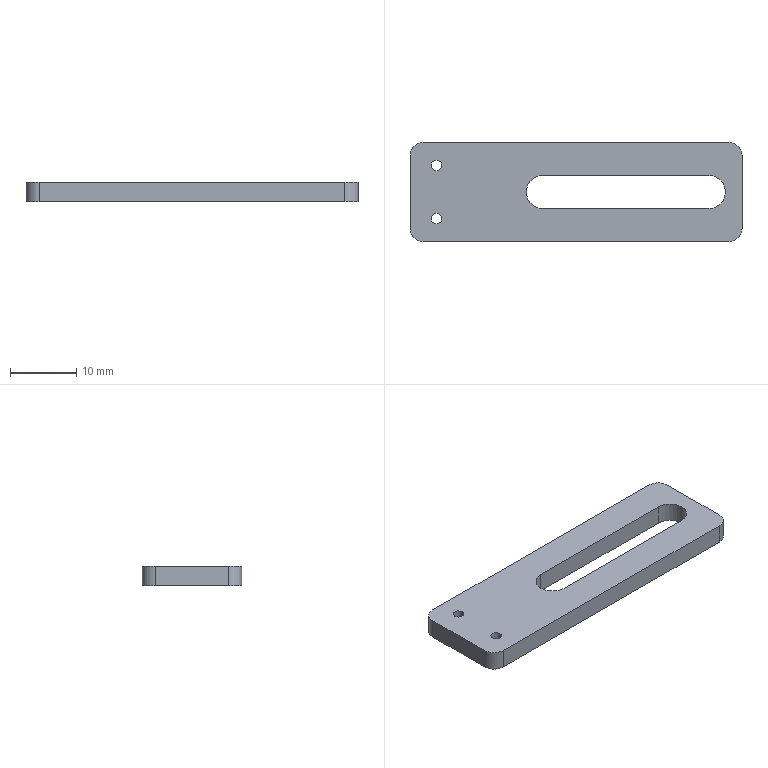Part | STEP file | 1004-2001-0085_1004-2001-0085_1-2 | 1 solid | 19 faces | box 50 x 15 x 3 mm | volume 1794 mm3 | cylinder 11 | plane 8 | commonest cylinder face diameters 1.6 x4 4 x4 5 x3
STEP:
#1=CARTESIAN_POINT('',(-20.2,-4.,1.5));
#2=VERTEX_POINT('',#1);
#3=CARTESIAN_POINT('',(-21.8,-4.,1.5));
#4=VERTEX_POINT('',#3);
#5=CARTESIAN_POINT('',(-21.,-4.,1.5));
#6=DIRECTION('',(0.,0.,-1.));
#7=DIRECTION('',(-1.,0.,0.));
#8=AXIS2_PLACEMENT_3D('',#5,#6,#7);
#9=CIRCLE('',#8,0.8);
#10=EDGE_CURVE('',#2,#4,#9,.T.);
#11=ORIENTED_EDGE('',*,*,#10,.F.);
#12=CARTESIAN_POINT('',(-20.2,-4.,-1.5));
#13=VERTEX_POINT('',#12);
#14=CARTESIAN_POINT('',(-20.2,-4.,-1.5));
#15=DIRECTION('',(0.,0.,-1.));
#16=VECTOR('',#15,1000.);
#17=LINE('',#14,#16);
#18=EDGE_CURVE('',#2,#13,#17,.T.);
#19=ORIENTED_EDGE('',*,*,#18,.T.);
#20=CARTESIAN_POINT('',(-21.8,-4.,-1.5));
#21=VERTEX_POINT('',#20);
#22=CARTESIAN_POINT('',(-21.,-4.,-1.5));
#23=DIRECTION('',(0.,0.,1.));
#24=DIRECTION('',(-1.,0.,0.));
#25=AXIS2_PLACEMENT_3D('',#22,#23,#24);
#26=CIRCLE('',#25,0.8);
#27=EDGE_CURVE('',#21,#13,#26,.T.);
#28=ORIENTED_EDGE('',*,*,#27,.F.);
#29=CARTESIAN_POINT('',(-21.8,-4.,-1.5));
#30=DIRECTION('',(0.,0.,-1.));
#31=VECTOR('',#30,1000.);
#32=LINE('',#29,#31);
#33=EDGE_CURVE('',#4,#21,#32,.T.);
#34=ORIENTED_EDGE('',*,*,#33,.F.);
#35=EDGE_LOOP('',(#11,#19,#28,#34));
#36=FACE_OUTER_BOUND('',#35,.T.);
#37=CARTESIAN_POINT('',(-21.,-4.,-1.5));
#38=DIRECTION('',(0.,0.,-1.));
#39=DIRECTION('',(-1.,0.,0.));
#40=AXIS2_PLACEMENT_3D('',#37,#38,#39);
#41=CYLINDRICAL_SURFACE('',#40,0.8);
#42=ADVANCED_FACE('',(#36),#41,.F.);
#43=CARTESIAN_POINT('',(-20.2,4.,1.5));
#44=VERTEX_POINT('',#43);
#45=CARTESIAN_POINT('',(-21.8,4.,1.5));
#46=VERTEX_POINT('',#45);
#47=CARTESIAN_POINT('',(-21.,4.,1.5));
#48=DIRECTION('',(0.,0.,-1.));
#49=DIRECTION('',(-1.,0.,0.));
#50=AXIS2_PLACEMENT_3D('',#47,#48,#49);
#51=CIRCLE('',#50,0.8);
#52=EDGE_CURVE('',#44,#46,#51,.T.);
#53=ORIENTED_EDGE('',*,*,#52,.F.);
#54=CARTESIAN_POINT('',(-20.2,4.,-1.5));
#55=VERTEX_POINT('',#54);
#56=CARTESIAN_POINT('',(-20.2,4.,-1.5));
#57=DIRECTION('',(0.,0.,-1.));
#58=VECTOR('',#57,1000.);
#59=LINE('',#56,#58);
#60=EDGE_CURVE('',#44,#55,#59,.T.);
#61=ORIENTED_EDGE('',*,*,#60,.T.);
#62=CARTESIAN_POINT('',(-21.8,4.,-1.5));
#63=VERTEX_POINT('',#62);
#64=CARTESIAN_POINT('',(-21.,4.,-1.5));
#65=DIRECTION('',(0.,0.,1.));
#66=DIRECTION('',(-1.,0.,0.));
#67=AXIS2_PLACEMENT_3D('',#64,#65,#66);
#68=CIRCLE('',#67,0.8);
#69=EDGE_CURVE('',#63,#55,#68,.T.);
#70=ORIENTED_EDGE('',*,*,#69,.F.);
#71=CARTESIAN_POINT('',(-21.8,4.,-1.5));
#72=DIRECTION('',(0.,0.,-1.));
#73=VECTOR('',#72,1000.);
#74=LINE('',#71,#73);
#75=EDGE_CURVE('',#46,#63,#74,.T.);
#76=ORIENTED_EDGE('',*,*,#75,.F.);
#77=EDGE_LOOP('',(#53,#61,#70,#76));
#78=FACE_OUTER_BOUND('',#77,.T.);
#79=CARTESIAN_POINT('',(-21.,4.,-1.5));
#80=DIRECTION('',(0.,0.,-1.));
#81=DIRECTION('',(-1.,0.,0.));
#82=AXIS2_PLACEMENT_3D('',#79,#80,#81);
#83=CYLINDRICAL_SURFACE('',#82,0.8);
#84=ADVANCED_FACE('',(#78),#83,.F.);
#85=CARTESIAN_POINT('',(-7.5,0.,1.5));
#86=VERTEX_POINT('',#85);
#87=CARTESIAN_POINT('',(-5.,2.5,1.5));
#88=VERTEX_POINT('',#87);
#89=CARTESIAN_POINT('',(-5.,0.,1.5));
#90=DIRECTION('',(0.,0.,-1.));
#91=DIRECTION('',(-1.,0.,0.));
#92=AXIS2_PLACEMENT_3D('',#89,#90,#91);
#93=CIRCLE('',#92,2.5);
#94=EDGE_CURVE('',#86,#88,#93,.T.);
#95=ORIENTED_EDGE('',*,*,#94,.F.);
#96=CARTESIAN_POINT('',(-7.5,0.,-1.5));
#97=VERTEX_POINT('',#96);
#98=CARTESIAN_POINT('',(-7.5,0.,1.5));
#99=DIRECTION('',(0.,0.,-1.));
#100=VECTOR('',#99,1000.);
#101=LINE('',#98,#100);
#102=EDGE_CURVE('',#86,#97,#101,.T.);
#103=ORIENTED_EDGE('',*,*,#102,.T.);
#104=CARTESIAN_POINT('',(-5.,2.5,-1.5));
#105=VERTEX_POINT('',#104);
#106=CARTESIAN_POINT('',(-5.,0.,-1.5));
#107=DIRECTION('',(0.,0.,1.));
#108=DIRECTION('',(-1.,0.,0.));
#109=AXIS2_PLACEMENT_3D('',#106,#107,#108);
#110=CIRCLE('',#109,2.5);
#111=EDGE_CURVE('',#105,#97,#110,.T.);
#112=ORIENTED_EDGE('',*,*,#111,.F.);
#113=CARTESIAN_POINT('',(-5.,2.5,1.5));
#114=DIRECTION('',(0.,0.,1.));
#115=VECTOR('',#114,1000.);
#116=LINE('',#113,#115);
#117=EDGE_CURVE('',#105,#88,#116,.T.);
#118=ORIENTED_EDGE('',*,*,#117,.T.);
#119=EDGE_LOOP('',(#95,#103,#112,#118));
#120=FACE_OUTER_BOUND('',#119,.T.);
#121=CARTESIAN_POINT('',(-5.,0.,1.5));
#122=DIRECTION('',(0.,0.,-1.));
#123=DIRECTION('',(-1.,0.,0.));
#124=AXIS2_PLACEMENT_3D('',#121,#122,#123);
#125=CYLINDRICAL_SURFACE('',#124,2.5);
#126=ADVANCED_FACE('',(#120),#125,.F.);
#127=CARTESIAN_POINT('',(-21.,-4.,1.5));
#128=DIRECTION('',(0.,0.,-1.));
#129=DIRECTION('',(-1.,0.,0.));
#130=AXIS2_PLACEMENT_3D('',#127,#128,#129);
#131=CIRCLE('',#130,0.8);
#132=EDGE_CURVE('',#4,#2,#131,.T.);
#133=ORIENTED_EDGE('',*,*,#132,.T.);
#134=ORIENTED_EDGE('',*,*,#10,.T.);
#135=EDGE_LOOP('',(#133,#134));
#136=FACE_BOUND('',#135,.T.);
#137=CARTESIAN_POINT('',(-21.,4.,1.5));
#138=DIRECTION('',(0.,0.,-1.));
#139=DIRECTION('',(-1.,0.,0.));
#140=AXIS2_PLACEMENT_3D('',#137,#138,#139);
#141=CIRCLE('',#140,0.8);
#142=EDGE_CURVE('',#46,#44,#141,.T.);
#143=ORIENTED_EDGE('',*,*,#142,.T.);
#144=ORIENTED_EDGE('',*,*,#52,.T.);
#145=EDGE_LOOP('',(#143,#144));
#146=FACE_BOUND('',#145,.T.);
#147=CARTESIAN_POINT('',(20.,-2.5,1.5));
#148=VERTEX_POINT('',#147);
#149=CARTESIAN_POINT('',(-5.,-2.5,1.5));
#150=VERTEX_POINT('',#149);
#151=CARTESIAN_POINT('',(-25.,-2.5,1.5));
#152=DIRECTION('',(-1.,0.,0.));
#153=VECTOR('',#152,1000.);
#154=LINE('',#151,#153);
#155=EDGE_CURVE('',#148,#150,#154,.T.);
#156=ORIENTED_EDGE('',*,*,#155,.T.);
#157=CARTESIAN_POINT('',(-5.,0.,1.5));
#158=DIRECTION('',(0.,0.,-1.));
#159=DIRECTION('',(-1.,0.,0.));
#160=AXIS2_PLACEMENT_3D('',#157,#158,#159);
#161=CIRCLE('',#160,2.5);
#162=EDGE_CURVE('',#150,#86,#161,.T.);
#163=ORIENTED_EDGE('',*,*,#162,.T.);
#164=ORIENTED_EDGE('',*,*,#94,.T.);
#165=CARTESIAN_POINT('',(20.,2.5,1.5));
#166=VERTEX_POINT('',#165);
#167=CARTESIAN_POINT('',(-25.,2.5,1.5));
#168=DIRECTION('',(1.,0.,0.));
#169=VECTOR('',#168,1000.);
#170=LINE('',#167,#169);
#171=EDGE_CURVE('',#88,#166,#170,.T.);
#172=ORIENTED_EDGE('',*,*,#171,.T.);
#173=CARTESIAN_POINT('',(20.,0.,1.5));
#174=DIRECTION('',(0.,0.,-1.));
#175=DIRECTION('',(-1.,0.,0.));
#176=AXIS2_PLACEMENT_3D('',#173,#174,#175);
#177=CIRCLE('',#176,2.5);
#178=EDGE_CURVE('',#166,#148,#177,.T.);
#179=ORIENTED_EDGE('',*,*,#178,.T.);
#180=EDGE_LOOP('',(#156,#163,#164,#172,#179));
#181=FACE_BOUND('',#180,.T.);
#182=CARTESIAN_POINT('',(23.,-7.5,1.5));
#183=VERTEX_POINT('',#182);
#184=CARTESIAN_POINT('',(25.,-5.5,1.5));
#185=VERTEX_POINT('',#184);
#186=CARTESIAN_POINT('',(23.,-5.5,1.5));
#187=DIRECTION('',(0.,0.,1.));
#188=DIRECTION('',(-1.,0.,0.));
#189=AXIS2_PLACEMENT_3D('',#186,#187,#188);
#190=CIRCLE('',#189,2.);
#191=EDGE_CURVE('',#183,#185,#190,.T.);
#192=ORIENTED_EDGE('',*,*,#191,.T.);
#193=CARTESIAN_POINT('',(25.,5.5,1.5));
#194=VERTEX_POINT('',#193);
#195=CARTESIAN_POINT('',(25.,7.5,1.5));
#196=DIRECTION('',(0.,1.,0.));
#197=VECTOR('',#196,1000.);
#198=LINE('',#195,#197);
#199=EDGE_CURVE('',#185,#194,#198,.T.);
#200=ORIENTED_EDGE('',*,*,#199,.T.);
#201=CARTESIAN_POINT('',(23.,7.5,1.5));
#202=VERTEX_POINT('',#201);
#203=CARTESIAN_POINT('',(23.,5.5,1.5));
#204=DIRECTION('',(0.,0.,1.));
#205=DIRECTION('',(-1.,0.,0.));
#206=AXIS2_PLACEMENT_3D('',#203,#204,#205);
#207=CIRCLE('',#206,2.);
#208=EDGE_CURVE('',#194,#202,#207,.T.);
#209=ORIENTED_EDGE('',*,*,#208,.T.);
#210=CARTESIAN_POINT('',(-23.,7.5,1.5));
#211=VERTEX_POINT('',#210);
#212=CARTESIAN_POINT('',(-25.,7.5,1.5));
#213=DIRECTION('',(-1.,0.,0.));
#214=VECTOR('',#213,1000.);
#215=LINE('',#212,#214);
#216=EDGE_CURVE('',#202,#211,#215,.T.);
#217=ORIENTED_EDGE('',*,*,#216,.T.);
#218=CARTESIAN_POINT('',(-25.,5.5,1.5));
#219=VERTEX_POINT('',#218);
#220=CARTESIAN_POINT('',(-23.,5.5,1.5));
#221=DIRECTION('',(0.,0.,1.));
#222=DIRECTION('',(-1.,0.,0.));
#223=AXIS2_PLACEMENT_3D('',#220,#221,#222);
#224=CIRCLE('',#223,2.);
#225=EDGE_CURVE('',#211,#219,#224,.T.);
#226=ORIENTED_EDGE('',*,*,#225,.T.);
#227=CARTESIAN_POINT('',(-25.,-5.5,1.5));
#228=VERTEX_POINT('',#227);
#229=CARTESIAN_POINT('',(-25.,7.5,1.5));
#230=DIRECTION('',(0.,-1.,0.));
#231=VECTOR('',#230,1000.);
#232=LINE('',#229,#231);
#233=EDGE_CURVE('',#219,#228,#232,.T.);
#234=ORIENTED_EDGE('',*,*,#233,.T.);
#235=CARTESIAN_POINT('',(-23.,-7.5,1.5));
#236=VERTEX_POINT('',#235);
#237=CARTESIAN_POINT('',(-23.,-5.5,1.5));
#238=DIRECTION('',(0.,0.,1.));
#239=DIRECTION('',(-1.,0.,0.));
#240=AXIS2_PLACEMENT_3D('',#237,#238,#239);
#241=CIRCLE('',#240,2.);
#242=EDGE_CURVE('',#228,#236,#241,.T.);
#243=ORIENTED_EDGE('',*,*,#242,.T.);
#244=CARTESIAN_POINT('',(-25.,-7.5,1.5));
#245=DIRECTION('',(1.,0.,0.));
#246=VECTOR('',#245,1000.);
#247=LINE('',#244,#246);
#248=EDGE_CURVE('',#236,#183,#247,.T.);
#249=ORIENTED_EDGE('',*,*,#248,.T.);
#250=EDGE_LOOP('',(#192,#200,#209,#217,#226,#234,#243,#249));
#251=FACE_OUTER_BOUND('',#250,.T.);
#252=CARTESIAN_POINT('',(-25.,7.5,1.5));
#253=DIRECTION('',(0.,0.,1.));
#254=DIRECTION('',(1.,0.,0.));
#255=AXIS2_PLACEMENT_3D('',#252,#253,#254);
#256=PLANE('',#255);
#257=ADVANCED_FACE('',(#136,#146,#181,#251),#256,.T.);
#258=ORIENTED_EDGE('',*,*,#18,.F.);
#259=ORIENTED_EDGE('',*,*,#132,.F.);
#260=ORIENTED_EDGE('',*,*,#33,.T.);
#261=CARTESIAN_POINT('',(-21.,-4.,-1.5));
#262=DIRECTION('',(0.,0.,1.));
#263=DIRECTION('',(-1.,0.,0.));
#264=AXIS2_PLACEMENT_3D('',#261,#262,#263);
#265=CIRCLE('',#264,0.8);
#266=EDGE_CURVE('',#13,#21,#265,.T.);
#267=ORIENTED_EDGE('',*,*,#266,.F.);
#268=EDGE_LOOP('',(#258,#259,#260,#267));
#269=FACE_OUTER_BOUND('',#268,.T.);
#270=CARTESIAN_POINT('',(-21.,-4.,-1.5));
#271=DIRECTION('',(0.,0.,-1.));
#272=DIRECTION('',(-1.,0.,0.));
#273=AXIS2_PLACEMENT_3D('',#270,#271,#272);
#274=CYLINDRICAL_SURFACE('',#273,0.8);
#275=ADVANCED_FACE('',(#269),#274,.F.);
#276=ORIENTED_EDGE('',*,*,#60,.F.);
#277=ORIENTED_EDGE('',*,*,#142,.F.);
#278=ORIENTED_EDGE('',*,*,#75,.T.);
#279=CARTESIAN_POINT('',(-21.,4.,-1.5));
#280=DIRECTION('',(0.,0.,1.));
#281=DIRECTION('',(-1.,0.,0.));
#282=AXIS2_PLACEMENT_3D('',#279,#280,#281);
#283=CIRCLE('',#282,0.8);
#284=EDGE_CURVE('',#55,#63,#283,.T.);
#285=ORIENTED_EDGE('',*,*,#284,.F.);
#286=EDGE_LOOP('',(#276,#277,#278,#285));
#287=FACE_OUTER_BOUND('',#286,.T.);
#288=CARTESIAN_POINT('',(-21.,4.,-1.5));
#289=DIRECTION('',(0.,0.,-1.));
#290=DIRECTION('',(-1.,0.,0.));
#291=AXIS2_PLACEMENT_3D('',#288,#289,#290);
#292=CYLINDRICAL_SURFACE('',#291,0.8);
#293=ADVANCED_FACE('',(#287),#292,.F.);
#294=ORIENTED_EDGE('',*,*,#102,.F.);
#295=ORIENTED_EDGE('',*,*,#162,.F.);
#296=CARTESIAN_POINT('',(-5.,-2.5,-1.5));
#297=VERTEX_POINT('',#296);
#298=CARTESIAN_POINT('',(-5.,-2.5,1.5));
#299=DIRECTION('',(0.,0.,1.));
#300=VECTOR('',#299,1000.);
#301=LINE('',#298,#300);
#302=EDGE_CURVE('',#297,#150,#301,.T.);
#303=ORIENTED_EDGE('',*,*,#302,.F.);
#304=CARTESIAN_POINT('',(-5.,0.,-1.5));
#305=DIRECTION('',(0.,0.,1.));
#306=DIRECTION('',(-1.,0.,0.));
#307=AXIS2_PLACEMENT_3D('',#304,#305,#306);
#308=CIRCLE('',#307,2.5);
#309=EDGE_CURVE('',#97,#297,#308,.T.);
#310=ORIENTED_EDGE('',*,*,#309,.F.);
#311=EDGE_LOOP('',(#294,#295,#303,#310));
#312=FACE_OUTER_BOUND('',#311,.T.);
#313=CARTESIAN_POINT('',(-5.,0.,1.5));
#314=DIRECTION('',(0.,0.,-1.));
#315=DIRECTION('',(-1.,0.,0.));
#316=AXIS2_PLACEMENT_3D('',#313,#314,#315);
#317=CYLINDRICAL_SURFACE('',#316,2.5);
#318=ADVANCED_FACE('',(#312),#317,.F.);
#319=ORIENTED_EDGE('',*,*,#155,.F.);
#320=CARTESIAN_POINT('',(20.,-2.5,-1.5));
#321=VERTEX_POINT('',#320);
#322=CARTESIAN_POINT('',(20.,-2.5,1.5));
#323=DIRECTION('',(0.,0.,1.));
#324=VECTOR('',#323,1000.);
#325=LINE('',#322,#324);
#326=EDGE_CURVE('',#321,#148,#325,.T.);
#327=ORIENTED_EDGE('',*,*,#326,.F.);
#328=CARTESIAN_POINT('',(-5.,-2.5,-1.5));
#329=DIRECTION('',(1.,0.,0.));
#330=VECTOR('',#329,1000.);
#331=LINE('',#328,#330);
#332=EDGE_CURVE('',#297,#321,#331,.T.);
#333=ORIENTED_EDGE('',*,*,#332,.F.);
#334=ORIENTED_EDGE('',*,*,#302,.T.);
#335=EDGE_LOOP('',(#319,#327,#333,#334));
#336=FACE_OUTER_BOUND('',#335,.T.);
#337=CARTESIAN_POINT('',(-5.,-2.5,1.5));
#338=DIRECTION('',(0.,-1.,0.));
#339=DIRECTION('',(0.,0.,-1.));
#340=AXIS2_PLACEMENT_3D('',#337,#338,#339);
#341=PLANE('',#340);
#342=ADVANCED_FACE('',(#336),#341,.F.);
#343=ORIENTED_EDGE('',*,*,#326,.T.);
#344=ORIENTED_EDGE('',*,*,#178,.F.);
#345=CARTESIAN_POINT('',(20.,2.5,-1.5));
#346=VERTEX_POINT('',#345);
#347=CARTESIAN_POINT('',(20.,2.5,1.5));
#348=DIRECTION('',(0.,0.,1.));
#349=VECTOR('',#348,1000.);
#350=LINE('',#347,#349);
#351=EDGE_CURVE('',#346,#166,#350,.T.);
#352=ORIENTED_EDGE('',*,*,#351,.F.);
#353=CARTESIAN_POINT('',(20.,0.,-1.5));
#354=DIRECTION('',(0.,0.,1.));
#355=DIRECTION('',(-1.,0.,0.));
#356=AXIS2_PLACEMENT_3D('',#353,#354,#355);
#357=CIRCLE('',#356,2.5);
#358=EDGE_CURVE('',#321,#346,#357,.T.);
#359=ORIENTED_EDGE('',*,*,#358,.F.);
#360=EDGE_LOOP('',(#343,#344,#352,#359));
#361=FACE_OUTER_BOUND('',#360,.T.);
#362=CARTESIAN_POINT('',(20.,0.,1.5));
#363=DIRECTION('',(0.,0.,-1.));
#364=DIRECTION('',(-1.,0.,0.));
#365=AXIS2_PLACEMENT_3D('',#362,#363,#364);
#366=CYLINDRICAL_SURFACE('',#365,2.5);
#367=ADVANCED_FACE('',(#361),#366,.F.);
#368=ORIENTED_EDGE('',*,*,#171,.F.);
#369=ORIENTED_EDGE('',*,*,#117,.F.);
#370=CARTESIAN_POINT('',(-5.,2.5,-1.5));
#371=DIRECTION('',(-1.,0.,0.));
#372=VECTOR('',#371,1000.);
#373=LINE('',#370,#372);
#374=EDGE_CURVE('',#346,#105,#373,.T.);
#375=ORIENTED_EDGE('',*,*,#374,.F.);
#376=ORIENTED_EDGE('',*,*,#351,.T.);
#377=EDGE_LOOP('',(#368,#369,#375,#376));
#378=FACE_OUTER_BOUND('',#377,.T.);
#379=CARTESIAN_POINT('',(-5.,2.5,1.5));
#380=DIRECTION('',(0.,1.,0.));
#381=DIRECTION('',(0.,0.,1.));
#382=AXIS2_PLACEMENT_3D('',#379,#380,#381);
#383=PLANE('',#382);
#384=ADVANCED_FACE('',(#378),#383,.F.);
#385=ORIENTED_EDGE('',*,*,#199,.F.);
#386=CARTESIAN_POINT('',(25.,-5.5,-1.5));
#387=VERTEX_POINT('',#386);
#388=CARTESIAN_POINT('',(25.,-5.5,1.5));
#389=DIRECTION('',(0.,0.,1.));
#390=VECTOR('',#389,1000.);
#391=LINE('',#388,#390);
#392=EDGE_CURVE('',#387,#185,#391,.T.);
#393=ORIENTED_EDGE('',*,*,#392,.F.);
#394=CARTESIAN_POINT('',(25.,5.5,-1.5));
#395=VERTEX_POINT('',#394);
#396=CARTESIAN_POINT('',(25.,-7.5,-1.5));
#397=DIRECTION('',(0.,-1.,0.));
#398=VECTOR('',#397,1000.);
#399=LINE('',#396,#398);
#400=EDGE_CURVE('',#395,#387,#399,.T.);
#401=ORIENTED_EDGE('',*,*,#400,.F.);
#402=CARTESIAN_POINT('',(25.,5.5,1.5));
#403=DIRECTION('',(0.,0.,-1.));
#404=VECTOR('',#403,1000.);
#405=LINE('',#402,#404);
#406=EDGE_CURVE('',#194,#395,#405,.T.);
#407=ORIENTED_EDGE('',*,*,#406,.F.);
#408=EDGE_LOOP('',(#385,#393,#401,#407));
#409=FACE_OUTER_BOUND('',#408,.T.);
#410=CARTESIAN_POINT('',(25.,-7.5,1.5));
#411=DIRECTION('',(-1.,0.,0.));
#412=DIRECTION('',(0.,0.,1.));
#413=AXIS2_PLACEMENT_3D('',#410,#411,#412);
#414=PLANE('',#413);
#415=ADVANCED_FACE('',(#409),#414,.F.);
#416=ORIENTED_EDGE('',*,*,#392,.T.);
#417=ORIENTED_EDGE('',*,*,#191,.F.);
#418=CARTESIAN_POINT('',(23.,-7.5,-1.5));
#419=VERTEX_POINT('',#418);
#420=CARTESIAN_POINT('',(23.,-7.5,1.5));
#421=DIRECTION('',(0.,0.,-1.));
#422=VECTOR('',#421,1000.);
#423=LINE('',#420,#422);
#424=EDGE_CURVE('',#183,#419,#423,.T.);
#425=ORIENTED_EDGE('',*,*,#424,.T.);
#426=CARTESIAN_POINT('',(23.,-5.5,-1.5));
#427=DIRECTION('',(0.,0.,1.));
#428=DIRECTION('',(-1.,0.,0.));
#429=AXIS2_PLACEMENT_3D('',#426,#427,#428);
#430=CIRCLE('',#429,2.);
#431=EDGE_CURVE('',#419,#387,#430,.T.);
#432=ORIENTED_EDGE('',*,*,#431,.T.);
#433=EDGE_LOOP('',(#416,#417,#425,#432));
#434=FACE_OUTER_BOUND('',#433,.T.);
#435=CARTESIAN_POINT('',(23.,-5.5,1.5));
#436=DIRECTION('',(0.,0.,-1.));
#437=DIRECTION('',(-1.,0.,0.));
#438=AXIS2_PLACEMENT_3D('',#435,#436,#437);
#439=CYLINDRICAL_SURFACE('',#438,2.);
#440=ADVANCED_FACE('',(#434),#439,.T.);
#441=ORIENTED_EDGE('',*,*,#248,.F.);
#442=CARTESIAN_POINT('',(-23.,-7.5,-1.5));
#443=VERTEX_POINT('',#442);
#444=CARTESIAN_POINT('',(-23.,-7.5,1.5));
#445=DIRECTION('',(0.,0.,1.));
#446=VECTOR('',#445,1000.);
#447=LINE('',#444,#446);
#448=EDGE_CURVE('',#443,#236,#447,.T.);
#449=ORIENTED_EDGE('',*,*,#448,.F.);
#450=CARTESIAN_POINT('',(25.,-7.5,-1.5));
#451=DIRECTION('',(-1.,0.,0.));
#452=VECTOR('',#451,1000.);
#453=LINE('',#450,#452);
#454=EDGE_CURVE('',#419,#443,#453,.T.);
#455=ORIENTED_EDGE('',*,*,#454,.F.);
#456=ORIENTED_EDGE('',*,*,#424,.F.);
#457=EDGE_LOOP('',(#441,#449,#455,#456));
#458=FACE_OUTER_BOUND('',#457,.T.);
#459=CARTESIAN_POINT('',(25.,-7.5,1.5));
#460=DIRECTION('',(0.,1.,0.));
#461=DIRECTION('',(0.,0.,1.));
#462=AXIS2_PLACEMENT_3D('',#459,#460,#461);
#463=PLANE('',#462);
#464=ADVANCED_FACE('',(#458),#463,.F.);
#465=ORIENTED_EDGE('',*,*,#448,.T.);
#466=ORIENTED_EDGE('',*,*,#242,.F.);
#467=CARTESIAN_POINT('',(-25.,-5.5,-1.5));
#468=VERTEX_POINT('',#467);
#469=CARTESIAN_POINT('',(-25.,-5.5,1.5));
#470=DIRECTION('',(0.,0.,-1.));
#471=VECTOR('',#470,1000.);
#472=LINE('',#469,#471);
#473=EDGE_CURVE('',#228,#468,#472,.T.);
#474=ORIENTED_EDGE('',*,*,#473,.T.);
#475=CARTESIAN_POINT('',(-23.,-5.5,-1.5));
#476=DIRECTION('',(0.,0.,1.));
#477=DIRECTION('',(-1.,0.,0.));
#478=AXIS2_PLACEMENT_3D('',#475,#476,#477);
#479=CIRCLE('',#478,2.);
#480=EDGE_CURVE('',#468,#443,#479,.T.);
#481=ORIENTED_EDGE('',*,*,#480,.T.);
#482=EDGE_LOOP('',(#465,#466,#474,#481));
#483=FACE_OUTER_BOUND('',#482,.T.);
#484=CARTESIAN_POINT('',(-23.,-5.5,1.5));
#485=DIRECTION('',(0.,0.,-1.));
#486=DIRECTION('',(-1.,0.,0.));
#487=AXIS2_PLACEMENT_3D('',#484,#485,#486);
#488=CYLINDRICAL_SURFACE('',#487,2.);
#489=ADVANCED_FACE('',(#483),#488,.T.);
#490=ORIENTED_EDGE('',*,*,#233,.F.);
#491=CARTESIAN_POINT('',(-25.,5.5,-1.5));
#492=VERTEX_POINT('',#491);
#493=CARTESIAN_POINT('',(-25.,5.5,1.5));
#494=DIRECTION('',(0.,0.,1.));
#495=VECTOR('',#494,1000.);
#496=LINE('',#493,#495);
#497=EDGE_CURVE('',#492,#219,#496,.T.);
#498=ORIENTED_EDGE('',*,*,#497,.F.);
#499=CARTESIAN_POINT('',(-25.,-7.5,-1.5));
#500=DIRECTION('',(0.,1.,0.));
#501=VECTOR('',#500,1000.);
#502=LINE('',#499,#501);
#503=EDGE_CURVE('',#468,#492,#502,.T.);
#504=ORIENTED_EDGE('',*,*,#503,.F.);
#505=ORIENTED_EDGE('',*,*,#473,.F.);
#506=EDGE_LOOP('',(#490,#498,#504,#505));
#507=FACE_OUTER_BOUND('',#506,.T.);
#508=CARTESIAN_POINT('',(-25.,-7.5,1.5));
#509=DIRECTION('',(1.,0.,0.));
#510=DIRECTION('',(0.,0.,-1.));
#511=AXIS2_PLACEMENT_3D('',#508,#509,#510);
#512=PLANE('',#511);
#513=ADVANCED_FACE('',(#507),#512,.F.);
#514=ORIENTED_EDGE('',*,*,#497,.T.);
#515=ORIENTED_EDGE('',*,*,#225,.F.);
#516=CARTESIAN_POINT('',(-23.,7.5,-1.5));
#517=VERTEX_POINT('',#516);
#518=CARTESIAN_POINT('',(-23.,7.5,1.5));
#519=DIRECTION('',(0.,0.,-1.));
#520=VECTOR('',#519,1000.);
#521=LINE('',#518,#520);
#522=EDGE_CURVE('',#211,#517,#521,.T.);
#523=ORIENTED_EDGE('',*,*,#522,.T.);
#524=CARTESIAN_POINT('',(-23.,5.5,-1.5));
#525=DIRECTION('',(0.,0.,1.));
#526=DIRECTION('',(-1.,0.,0.));
#527=AXIS2_PLACEMENT_3D('',#524,#525,#526);
#528=CIRCLE('',#527,2.);
#529=EDGE_CURVE('',#517,#492,#528,.T.);
#530=ORIENTED_EDGE('',*,*,#529,.T.);
#531=EDGE_LOOP('',(#514,#515,#523,#530));
#532=FACE_OUTER_BOUND('',#531,.T.);
#533=CARTESIAN_POINT('',(-23.,5.5,1.5));
#534=DIRECTION('',(0.,0.,-1.));
#535=DIRECTION('',(-1.,0.,0.));
#536=AXIS2_PLACEMENT_3D('',#533,#534,#535);
#537=CYLINDRICAL_SURFACE('',#536,2.);
#538=ADVANCED_FACE('',(#532),#537,.T.);
#539=CARTESIAN_POINT('',(23.,7.5,-1.5));
#540=VERTEX_POINT('',#539);
#541=CARTESIAN_POINT('',(25.,7.5,-1.5));
#542=DIRECTION('',(1.,0.,0.));
#543=VECTOR('',#542,1000.);
#544=LINE('',#541,#543);
#545=EDGE_CURVE('',#517,#540,#544,.T.);
#546=ORIENTED_EDGE('',*,*,#545,.F.);
#547=ORIENTED_EDGE('',*,*,#522,.F.);
#548=ORIENTED_EDGE('',*,*,#216,.F.);
#549=CARTESIAN_POINT('',(23.,7.5,1.5));
#550=DIRECTION('',(0.,0.,1.));
#551=VECTOR('',#550,1000.);
#552=LINE('',#549,#551);
#553=EDGE_CURVE('',#540,#202,#552,.T.);
#554=ORIENTED_EDGE('',*,*,#553,.F.);
#555=EDGE_LOOP('',(#546,#547,#548,#554));
#556=FACE_OUTER_BOUND('',#555,.T.);
#557=CARTESIAN_POINT('',(25.,7.5,1.5));
#558=DIRECTION('',(0.,-1.,0.));
#559=DIRECTION('',(0.,0.,-1.));
#560=AXIS2_PLACEMENT_3D('',#557,#558,#559);
#561=PLANE('',#560);
#562=ADVANCED_FACE('',(#556),#561,.F.);
#563=ORIENTED_EDGE('',*,*,#553,.T.);
#564=ORIENTED_EDGE('',*,*,#208,.F.);
#565=ORIENTED_EDGE('',*,*,#406,.T.);
#566=CARTESIAN_POINT('',(23.,5.5,-1.5));
#567=DIRECTION('',(0.,0.,1.));
#568=DIRECTION('',(-1.,0.,0.));
#569=AXIS2_PLACEMENT_3D('',#566,#567,#568);
#570=CIRCLE('',#569,2.);
#571=EDGE_CURVE('',#395,#540,#570,.T.);
#572=ORIENTED_EDGE('',*,*,#571,.T.);
#573=EDGE_LOOP('',(#563,#564,#565,#572));
#574=FACE_OUTER_BOUND('',#573,.T.);
#575=CARTESIAN_POINT('',(23.,5.5,1.5));
#576=DIRECTION('',(0.,0.,-1.));
#577=DIRECTION('',(-1.,0.,0.));
#578=AXIS2_PLACEMENT_3D('',#575,#576,#577);
#579=CYLINDRICAL_SURFACE('',#578,2.);
#580=ADVANCED_FACE('',(#574),#579,.T.);
#581=ORIENTED_EDGE('',*,*,#27,.T.);
#582=ORIENTED_EDGE('',*,*,#266,.T.);
#583=EDGE_LOOP('',(#581,#582));
#584=FACE_BOUND('',#583,.T.);
#585=ORIENTED_EDGE('',*,*,#69,.T.);
#586=ORIENTED_EDGE('',*,*,#284,.T.);
#587=EDGE_LOOP('',(#585,#586));
#588=FACE_BOUND('',#587,.T.);
#589=ORIENTED_EDGE('',*,*,#111,.T.);
#590=ORIENTED_EDGE('',*,*,#309,.T.);
#591=ORIENTED_EDGE('',*,*,#332,.T.);
#592=ORIENTED_EDGE('',*,*,#358,.T.);
#593=ORIENTED_EDGE('',*,*,#374,.T.);
#594=EDGE_LOOP('',(#589,#590,#591,#592,#593));
#595=FACE_BOUND('',#594,.T.);
#596=ORIENTED_EDGE('',*,*,#400,.T.);
#597=ORIENTED_EDGE('',*,*,#431,.F.);
#598=ORIENTED_EDGE('',*,*,#454,.T.);
#599=ORIENTED_EDGE('',*,*,#480,.F.);
#600=ORIENTED_EDGE('',*,*,#503,.T.);
#601=ORIENTED_EDGE('',*,*,#529,.F.);
#602=ORIENTED_EDGE('',*,*,#545,.T.);
#603=ORIENTED_EDGE('',*,*,#571,.F.);
#604=EDGE_LOOP('',(#596,#597,#598,#599,#600,#601,#602,#603));
#605=FACE_OUTER_BOUND('',#604,.T.);
#606=CARTESIAN_POINT('',(-25.,7.5,-1.5));
#607=DIRECTION('',(0.,0.,1.));
#608=DIRECTION('',(1.,0.,0.));
#609=AXIS2_PLACEMENT_3D('',#606,#607,#608);
#610=PLANE('',#609);
#611=ADVANCED_FACE('',(#584,#588,#595,#605),#610,.F.);
#612=CLOSED_SHELL('',(#42,#84,#126,#257,#275,#293,#318,#342,#367,#384,#415,#440,#464,#489,#513,#538,#562,#580,#611));
#613=MANIFOLD_SOLID_BREP('',#612);
#614=CARTESIAN_POINT('',(0.,0.,0.));
#615=DIRECTION('',(0.,0.,1.));
#616=DIRECTION('',(1.,0.,0.));
#617=AXIS2_PLACEMENT_3D('',#614,#615,#616);
#618=(LENGTH_UNIT()NAMED_UNIT(*)SI_UNIT(.MILLI.,.METRE.));
#619=UNCERTAINTY_MEASURE_WITH_UNIT(LENGTH_MEASURE(0.00001),#618,'','');
#620=(NAMED_UNIT(*)PLANE_ANGLE_UNIT()SI_UNIT($,.RADIAN.));
#621=(NAMED_UNIT(*)SI_UNIT($,.STERADIAN.)SOLID_ANGLE_UNIT());
#622=(GEOMETRIC_REPRESENTATION_CONTEXT(3)GLOBAL_UNCERTAINTY_ASSIGNED_CONTEXT((#619))GLOBAL_UNIT_ASSIGNED_CONTEXT((#618,#620,#621))REPRESENTATION_CONTEXT('',''));
#623=ADVANCED_BREP_SHAPE_REPRESENTATION('',(#613,#617),#622);